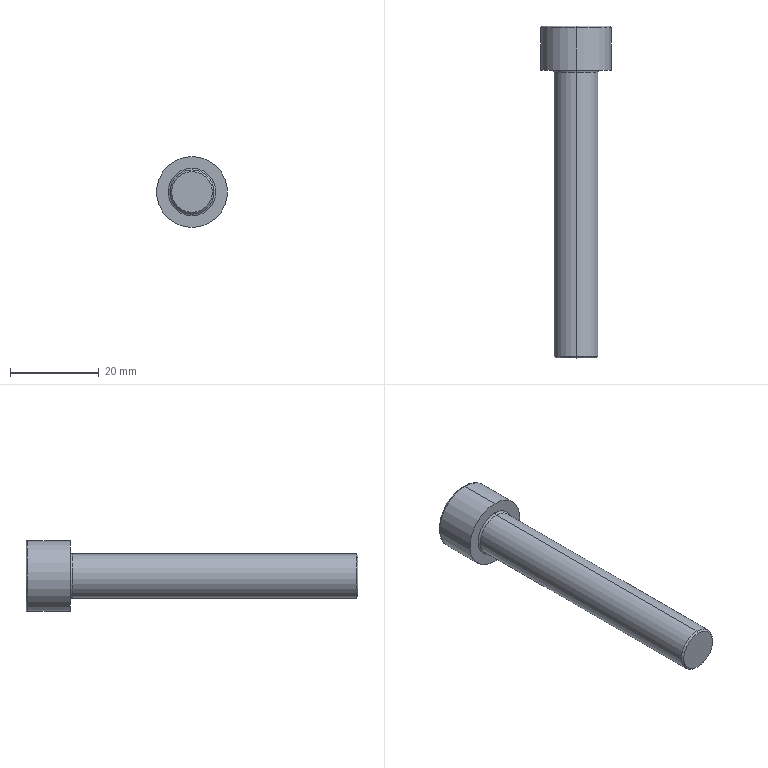Part | STEP file | 1 solid | 20 faces | box 16 x 75 x 16 mm | volume 6836 mm3 | plane 10 | torus 4 | cylinder 4 | cone 2 | commonest cylinder face diameters 10 x2 16 x2
STEP:
#1=CARTESIAN_POINT('',(0.,-65.,-4.6));
#2=VERTEX_POINT('',#1);
#3=CARTESIAN_POINT('',(0.,-65.,4.6));
#4=VERTEX_POINT('',#3);
#5=CARTESIAN_POINT('',(0.,-65.,0.));
#6=DIRECTION('',(0.,-1.,0.));
#7=DIRECTION('',(0.,0.,-1.));
#8=AXIS2_PLACEMENT_3D('',#5,#6,#7);
#9=CIRCLE('',#8,4.6);
#10=EDGE_CURVE('',#2,#4,#9,.T.);
#11=ORIENTED_EDGE('',*,*,#10,.F.);
#12=CARTESIAN_POINT('',(0.,-64.6,-5.));
#13=VERTEX_POINT('',#12);
#14=CARTESIAN_POINT('',(0.,-65.,-4.6));
#15=DIRECTION('',(0.,0.7071,-0.7071));
#16=VECTOR('',#15,1000.);
#17=LINE('',#14,#16);
#18=EDGE_CURVE('',#2,#13,#17,.T.);
#19=ORIENTED_EDGE('',*,*,#18,.T.);
#20=CARTESIAN_POINT('',(0.,-64.6,5.));
#21=VERTEX_POINT('',#20);
#22=CARTESIAN_POINT('',(0.,-64.6,0.));
#23=DIRECTION('',(0.,1.,0.));
#24=DIRECTION('',(0.,0.,-1.));
#25=AXIS2_PLACEMENT_3D('',#22,#23,#24);
#26=CIRCLE('',#25,5.);
#27=EDGE_CURVE('',#21,#13,#26,.T.);
#28=ORIENTED_EDGE('',*,*,#27,.F.);
#29=CARTESIAN_POINT('',(0.,-65.,4.6));
#30=DIRECTION('',(0.,0.7071,0.7071));
#31=VECTOR('',#30,1000.);
#32=LINE('',#29,#31);
#33=EDGE_CURVE('',#4,#21,#32,.T.);
#34=ORIENTED_EDGE('',*,*,#33,.F.);
#35=EDGE_LOOP('',(#11,#19,#28,#34));
#36=FACE_OUTER_BOUND('',#35,.T.);
#37=CARTESIAN_POINT('',(0.,-65.,0.));
#38=DIRECTION('',(0.,1.,0.));
#39=DIRECTION('',(0.,0.,1.));
#40=AXIS2_PLACEMENT_3D('',#37,#38,#39);
#41=CONICAL_SURFACE('',#40,4.6,0.7854);
#42=ADVANCED_FACE('',(#36),#41,.T.);
#43=CARTESIAN_POINT('',(0.,9.6,-8.));
#44=VERTEX_POINT('',#43);
#45=CARTESIAN_POINT('',(0.,9.6,8.));
#46=VERTEX_POINT('',#45);
#47=CARTESIAN_POINT('',(0.,9.6,0.));
#48=DIRECTION('',(0.,-1.,0.));
#49=DIRECTION('',(0.,0.,1.));
#50=AXIS2_PLACEMENT_3D('',#47,#48,#49);
#51=CIRCLE('',#50,8.);
#52=EDGE_CURVE('',#44,#46,#51,.T.);
#53=ORIENTED_EDGE('',*,*,#52,.F.);
#54=CARTESIAN_POINT('',(0.,10.,-7.6));
#55=VERTEX_POINT('',#54);
#56=CARTESIAN_POINT('',(0.,9.6,-7.6));
#57=DIRECTION('',(1.,0.,0.));
#58=DIRECTION('',(0.,0.,-1.));
#59=AXIS2_PLACEMENT_3D('',#56,#57,#58);
#60=CIRCLE('',#59,0.4);
#61=EDGE_CURVE('',#44,#55,#60,.T.);
#62=ORIENTED_EDGE('',*,*,#61,.T.);
#63=CARTESIAN_POINT('',(0.,10.,7.6));
#64=VERTEX_POINT('',#63);
#65=CARTESIAN_POINT('',(0.,10.,0.));
#66=DIRECTION('',(0.,1.,0.));
#67=DIRECTION('',(0.,0.,1.));
#68=AXIS2_PLACEMENT_3D('',#65,#66,#67);
#69=CIRCLE('',#68,7.6);
#70=EDGE_CURVE('',#64,#55,#69,.T.);
#71=ORIENTED_EDGE('',*,*,#70,.F.);
#72=CARTESIAN_POINT('',(0.,9.6,7.6));
#73=DIRECTION('',(-1.,0.,0.));
#74=DIRECTION('',(0.,0.,1.));
#75=AXIS2_PLACEMENT_3D('',#72,#73,#74);
#76=CIRCLE('',#75,0.4);
#77=EDGE_CURVE('',#46,#64,#76,.T.);
#78=ORIENTED_EDGE('',*,*,#77,.F.);
#79=EDGE_LOOP('',(#53,#62,#71,#78));
#80=FACE_OUTER_BOUND('',#79,.T.);
#81=CARTESIAN_POINT('',(0.,9.6,0.));
#82=DIRECTION('',(0.,1.,0.));
#83=DIRECTION('',(0.,0.,1.));
#84=AXIS2_PLACEMENT_3D('',#81,#82,#83);
#85=TOROIDAL_SURFACE('',#84,7.6,0.4);
#86=ADVANCED_FACE('',(#80),#85,.T.);
#87=CARTESIAN_POINT('',(0.,-0.4,5.));
#88=VERTEX_POINT('',#87);
#89=CARTESIAN_POINT('',(0.,-0.4,-5.));
#90=VERTEX_POINT('',#89);
#91=CARTESIAN_POINT('',(0.,-0.4,0.));
#92=DIRECTION('',(0.,-1.,0.));
#93=DIRECTION('',(0.,0.,-1.));
#94=AXIS2_PLACEMENT_3D('',#91,#92,#93);
#95=CIRCLE('',#94,5.);
#96=EDGE_CURVE('',#88,#90,#95,.T.);
#97=ORIENTED_EDGE('',*,*,#96,.F.);
#98=CARTESIAN_POINT('',(0.,0.,5.4));
#99=VERTEX_POINT('',#98);
#100=CARTESIAN_POINT('',(0.,-0.4,5.4));
#101=DIRECTION('',(1.,0.,0.));
#102=DIRECTION('',(0.,0.,-1.));
#103=AXIS2_PLACEMENT_3D('',#100,#101,#102);
#104=CIRCLE('',#103,0.4);
#105=EDGE_CURVE('',#88,#99,#104,.T.);
#106=ORIENTED_EDGE('',*,*,#105,.T.);
#107=CARTESIAN_POINT('',(0.,0.,-5.4));
#108=VERTEX_POINT('',#107);
#109=CARTESIAN_POINT('',(0.,0.,0.));
#110=DIRECTION('',(0.,1.,0.));
#111=DIRECTION('',(0.,0.,-1.));
#112=AXIS2_PLACEMENT_3D('',#109,#110,#111);
#113=CIRCLE('',#112,5.4);
#114=EDGE_CURVE('',#108,#99,#113,.T.);
#115=ORIENTED_EDGE('',*,*,#114,.F.);
#116=CARTESIAN_POINT('',(0.,-0.4,-5.4));
#117=DIRECTION('',(-1.,0.,0.));
#118=DIRECTION('',(0.,0.,1.));
#119=AXIS2_PLACEMENT_3D('',#116,#117,#118);
#120=CIRCLE('',#119,0.4);
#121=EDGE_CURVE('',#90,#108,#120,.T.);
#122=ORIENTED_EDGE('',*,*,#121,.F.);
#123=EDGE_LOOP('',(#97,#106,#115,#122));
#124=FACE_OUTER_BOUND('',#123,.T.);
#125=CARTESIAN_POINT('',(0.,-0.4,0.));
#126=DIRECTION('',(0.,-1.,0.));
#127=DIRECTION('',(0.,0.,-1.));
#128=AXIS2_PLACEMENT_3D('',#125,#126,#127);
#129=TOROIDAL_SURFACE('',#128,5.4,0.4);
#130=ADVANCED_FACE('',(#124),#129,.F.);
#131=CARTESIAN_POINT('',(0.,-0.4,0.));
#132=DIRECTION('',(0.,-1.,0.));
#133=DIRECTION('',(0.,0.,-1.));
#134=AXIS2_PLACEMENT_3D('',#131,#132,#133);
#135=CIRCLE('',#134,5.);
#136=EDGE_CURVE('',#90,#88,#135,.T.);
#137=ORIENTED_EDGE('',*,*,#136,.T.);
#138=CARTESIAN_POINT('',(0.,0.,5.));
#139=DIRECTION('',(0.,-1.,0.));
#140=VECTOR('',#139,1000.);
#141=LINE('',#138,#140);
#142=EDGE_CURVE('',#88,#21,#141,.T.);
#143=ORIENTED_EDGE('',*,*,#142,.T.);
#144=ORIENTED_EDGE('',*,*,#27,.T.);
#145=CARTESIAN_POINT('',(0.,0.,-5.));
#146=DIRECTION('',(0.,-1.,0.));
#147=VECTOR('',#146,1000.);
#148=LINE('',#145,#147);
#149=EDGE_CURVE('',#90,#13,#148,.T.);
#150=ORIENTED_EDGE('',*,*,#149,.F.);
#151=EDGE_LOOP('',(#137,#143,#144,#150));
#152=FACE_OUTER_BOUND('',#151,.T.);
#153=CARTESIAN_POINT('',(0.,0.,0.));
#154=DIRECTION('',(0.,-1.,0.));
#155=DIRECTION('',(0.,0.,-1.));
#156=AXIS2_PLACEMENT_3D('',#153,#154,#155);
#157=CYLINDRICAL_SURFACE('',#156,5.);
#158=ADVANCED_FACE('',(#152),#157,.T.);
#159=ORIENTED_EDGE('',*,*,#52,.T.);
#160=CARTESIAN_POINT('',(0.,0.,8.));
#161=VERTEX_POINT('',#160);
#162=CARTESIAN_POINT('',(0.,0.,8.));
#163=DIRECTION('',(0.,-1.,0.));
#164=VECTOR('',#163,1000.);
#165=LINE('',#162,#164);
#166=EDGE_CURVE('',#46,#161,#165,.T.);
#167=ORIENTED_EDGE('',*,*,#166,.T.);
#168=CARTESIAN_POINT('',(0.,0.,-8.));
#169=VERTEX_POINT('',#168);
#170=CARTESIAN_POINT('',(0.,0.,0.));
#171=DIRECTION('',(0.,-1.,0.));
#172=DIRECTION('',(0.,0.,-1.));
#173=AXIS2_PLACEMENT_3D('',#170,#171,#172);
#174=CIRCLE('',#173,8.);
#175=EDGE_CURVE('',#169,#161,#174,.T.);
#176=ORIENTED_EDGE('',*,*,#175,.F.);
#177=CARTESIAN_POINT('',(0.,0.,-8.));
#178=DIRECTION('',(0.,-1.,0.));
#179=VECTOR('',#178,1000.);
#180=LINE('',#177,#179);
#181=EDGE_CURVE('',#44,#169,#180,.T.);
#182=ORIENTED_EDGE('',*,*,#181,.F.);
#183=EDGE_LOOP('',(#159,#167,#176,#182));
#184=FACE_OUTER_BOUND('',#183,.T.);
#185=CARTESIAN_POINT('',(0.,0.,0.));
#186=DIRECTION('',(0.,-1.,0.));
#187=DIRECTION('',(0.,0.,-1.));
#188=AXIS2_PLACEMENT_3D('',#185,#186,#187);
#189=CYLINDRICAL_SURFACE('',#188,8.);
#190=ADVANCED_FACE('',(#184),#189,.T.);
#191=ORIENTED_EDGE('',*,*,#70,.T.);
#192=CARTESIAN_POINT('',(0.,10.,0.));
#193=DIRECTION('',(0.,1.,0.));
#194=DIRECTION('',(0.,0.,1.));
#195=AXIS2_PLACEMENT_3D('',#192,#193,#194);
#196=CIRCLE('',#195,7.6);
#197=EDGE_CURVE('',#55,#64,#196,.T.);
#198=ORIENTED_EDGE('',*,*,#197,.T.);
#199=EDGE_LOOP('',(#191,#198));
#200=FACE_OUTER_BOUND('',#199,.T.);
#201=CARTESIAN_POINT('',(0.,10.,-4.619));
#202=VERTEX_POINT('',#201);
#203=CARTESIAN_POINT('',(-4.,10.,-2.309));
#204=VERTEX_POINT('',#203);
#205=CARTESIAN_POINT('',(0.,10.,-4.619));
#206=DIRECTION('',(-0.866,0.,0.5));
#207=VECTOR('',#206,1000.);
#208=LINE('',#205,#207);
#209=EDGE_CURVE('',#202,#204,#208,.T.);
#210=ORIENTED_EDGE('',*,*,#209,.F.);
#211=CARTESIAN_POINT('',(4.,10.,-2.309));
#212=VERTEX_POINT('',#211);
#213=CARTESIAN_POINT('',(4.,10.,-2.309));
#214=DIRECTION('',(-0.866,0.,-0.5));
#215=VECTOR('',#214,1000.);
#216=LINE('',#213,#215);
#217=EDGE_CURVE('',#212,#202,#216,.T.);
#218=ORIENTED_EDGE('',*,*,#217,.F.);
#219=CARTESIAN_POINT('',(4.,10.,2.309));
#220=VERTEX_POINT('',#219);
#221=CARTESIAN_POINT('',(4.,10.,2.309));
#222=DIRECTION('',(0.,0.,-1.));
#223=VECTOR('',#222,1000.);
#224=LINE('',#221,#223);
#225=EDGE_CURVE('',#220,#212,#224,.T.);
#226=ORIENTED_EDGE('',*,*,#225,.F.);
#227=CARTESIAN_POINT('',(0.,10.,4.619));
#228=VERTEX_POINT('',#227);
#229=CARTESIAN_POINT('',(0.,10.,4.619));
#230=DIRECTION('',(0.866,0.,-0.5));
#231=VECTOR('',#230,1000.);
#232=LINE('',#229,#231);
#233=EDGE_CURVE('',#228,#220,#232,.T.);
#234=ORIENTED_EDGE('',*,*,#233,.F.);
#235=CARTESIAN_POINT('',(-4.,10.,2.309));
#236=VERTEX_POINT('',#235);
#237=CARTESIAN_POINT('',(-4.,10.,2.309));
#238=DIRECTION('',(0.866,0.,0.5));
#239=VECTOR('',#238,1000.);
#240=LINE('',#237,#239);
#241=EDGE_CURVE('',#236,#228,#240,.T.);
#242=ORIENTED_EDGE('',*,*,#241,.F.);
#243=CARTESIAN_POINT('',(-4.,10.,-2.309));
#244=DIRECTION('',(0.,0.,1.));
#245=VECTOR('',#244,1000.);
#246=LINE('',#243,#245);
#247=EDGE_CURVE('',#204,#236,#246,.T.);
#248=ORIENTED_EDGE('',*,*,#247,.F.);
#249=EDGE_LOOP('',(#210,#218,#226,#234,#242,#248));
#250=FACE_BOUND('',#249,.T.);
#251=CARTESIAN_POINT('',(0.,10.,0.));
#252=DIRECTION('',(0.,1.,0.));
#253=DIRECTION('',(0.,0.,1.));
#254=AXIS2_PLACEMENT_3D('',#251,#252,#253);
#255=PLANE('',#254);
#256=ADVANCED_FACE('',(#200,#250),#255,.T.);
#257=ORIENTED_EDGE('',*,*,#166,.F.);
#258=CARTESIAN_POINT('',(0.,9.6,0.));
#259=DIRECTION('',(0.,-1.,0.));
#260=DIRECTION('',(0.,0.,1.));
#261=AXIS2_PLACEMENT_3D('',#258,#259,#260);
#262=CIRCLE('',#261,8.);
#263=EDGE_CURVE('',#46,#44,#262,.T.);
#264=ORIENTED_EDGE('',*,*,#263,.T.);
#265=ORIENTED_EDGE('',*,*,#181,.T.);
#266=CARTESIAN_POINT('',(0.,0.,0.));
#267=DIRECTION('',(0.,-1.,0.));
#268=DIRECTION('',(0.,0.,-1.));
#269=AXIS2_PLACEMENT_3D('',#266,#267,#268);
#270=CIRCLE('',#269,8.);
#271=EDGE_CURVE('',#161,#169,#270,.T.);
#272=ORIENTED_EDGE('',*,*,#271,.F.);
#273=EDGE_LOOP('',(#257,#264,#265,#272));
#274=FACE_OUTER_BOUND('',#273,.T.);
#275=CARTESIAN_POINT('',(0.,0.,0.));
#276=DIRECTION('',(0.,-1.,0.));
#277=DIRECTION('',(0.,0.,-1.));
#278=AXIS2_PLACEMENT_3D('',#275,#276,#277);
#279=CYLINDRICAL_SURFACE('',#278,8.);
#280=ADVANCED_FACE('',(#274),#279,.T.);
#281=ORIENTED_EDGE('',*,*,#114,.T.);
#282=CARTESIAN_POINT('',(0.,0.,0.));
#283=DIRECTION('',(0.,1.,0.));
#284=DIRECTION('',(0.,0.,-1.));
#285=AXIS2_PLACEMENT_3D('',#282,#283,#284);
#286=CIRCLE('',#285,5.4);
#287=EDGE_CURVE('',#99,#108,#286,.T.);
#288=ORIENTED_EDGE('',*,*,#287,.T.);
#289=EDGE_LOOP('',(#281,#288));
#290=FACE_BOUND('',#289,.T.);
#291=ORIENTED_EDGE('',*,*,#175,.T.);
#292=ORIENTED_EDGE('',*,*,#271,.T.);
#293=EDGE_LOOP('',(#291,#292));
#294=FACE_OUTER_BOUND('',#293,.T.);
#295=CARTESIAN_POINT('',(8.,0.,0.));
#296=DIRECTION('',(0.,-1.,0.));
#297=DIRECTION('',(0.,0.,-1.));
#298=AXIS2_PLACEMENT_3D('',#295,#296,#297);
#299=PLANE('',#298);
#300=ADVANCED_FACE('',(#290,#294),#299,.T.);
#301=ORIENTED_EDGE('',*,*,#142,.F.);
#302=ORIENTED_EDGE('',*,*,#96,.T.);
#303=ORIENTED_EDGE('',*,*,#149,.T.);
#304=CARTESIAN_POINT('',(0.,-64.6,0.));
#305=DIRECTION('',(0.,1.,0.));
#306=DIRECTION('',(0.,0.,-1.));
#307=AXIS2_PLACEMENT_3D('',#304,#305,#306);
#308=CIRCLE('',#307,5.);
#309=EDGE_CURVE('',#13,#21,#308,.T.);
#310=ORIENTED_EDGE('',*,*,#309,.T.);
#311=EDGE_LOOP('',(#301,#302,#303,#310));
#312=FACE_OUTER_BOUND('',#311,.T.);
#313=CARTESIAN_POINT('',(0.,0.,0.));
#314=DIRECTION('',(0.,-1.,0.));
#315=DIRECTION('',(0.,0.,-1.));
#316=AXIS2_PLACEMENT_3D('',#313,#314,#315);
#317=CYLINDRICAL_SURFACE('',#316,5.);
#318=ADVANCED_FACE('',(#312),#317,.T.);
#319=CARTESIAN_POINT('',(0.,-65.,0.));
#320=DIRECTION('',(0.,-1.,0.));
#321=DIRECTION('',(0.,0.,-1.));
#322=AXIS2_PLACEMENT_3D('',#319,#320,#321);
#323=CIRCLE('',#322,4.6);
#324=EDGE_CURVE('',#4,#2,#323,.T.);
#325=ORIENTED_EDGE('',*,*,#324,.T.);
#326=ORIENTED_EDGE('',*,*,#10,.T.);
#327=EDGE_LOOP('',(#325,#326));
#328=FACE_OUTER_BOUND('',#327,.T.);
#329=CARTESIAN_POINT('',(5.,-65.,0.));
#330=DIRECTION('',(0.,-1.,0.));
#331=DIRECTION('',(0.,0.,-1.));
#332=AXIS2_PLACEMENT_3D('',#329,#330,#331);
#333=PLANE('',#332);
#334=ADVANCED_FACE('',(#328),#333,.T.);
#335=ORIENTED_EDGE('',*,*,#209,.T.);
#336=CARTESIAN_POINT('',(-4.,5.,-2.309));
#337=VERTEX_POINT('',#336);
#338=CARTESIAN_POINT('',(-4.,5.,-2.309));
#339=DIRECTION('',(0.,1.,0.));
#340=VECTOR('',#339,1000.);
#341=LINE('',#338,#340);
#342=EDGE_CURVE('',#337,#204,#341,.T.);
#343=ORIENTED_EDGE('',*,*,#342,.F.);
#344=CARTESIAN_POINT('',(0.,5.,-4.619));
#345=VERTEX_POINT('',#344);
#346=CARTESIAN_POINT('',(0.,5.,-4.619));
#347=DIRECTION('',(-0.866,0.,0.5));
#348=VECTOR('',#347,1000.);
#349=LINE('',#346,#348);
#350=EDGE_CURVE('',#345,#337,#349,.T.);
#351=ORIENTED_EDGE('',*,*,#350,.F.);
#352=CARTESIAN_POINT('',(0.,5.,-4.619));
#353=DIRECTION('',(0.,1.,0.));
#354=VECTOR('',#353,1000.);
#355=LINE('',#352,#354);
#356=EDGE_CURVE('',#345,#202,#355,.T.);
#357=ORIENTED_EDGE('',*,*,#356,.T.);
#358=EDGE_LOOP('',(#335,#343,#351,#357));
#359=FACE_OUTER_BOUND('',#358,.T.);
#360=CARTESIAN_POINT('',(0.,5.,-4.619));
#361=DIRECTION('',(-0.5,0.,-0.866));
#362=DIRECTION('',(-0.866,0.,0.5));
#363=AXIS2_PLACEMENT_3D('',#360,#361,#362);
#364=PLANE('',#363);
#365=ADVANCED_FACE('',(#359),#364,.F.);
#366=ORIENTED_EDGE('',*,*,#217,.T.);
#367=ORIENTED_EDGE('',*,*,#356,.F.);
#368=CARTESIAN_POINT('',(4.,5.,-2.309));
#369=VERTEX_POINT('',#368);
#370=CARTESIAN_POINT('',(4.,5.,-2.309));
#371=DIRECTION('',(-0.866,0.,-0.5));
#372=VECTOR('',#371,1000.);
#373=LINE('',#370,#372);
#374=EDGE_CURVE('',#369,#345,#373,.T.);
#375=ORIENTED_EDGE('',*,*,#374,.F.);
#376=CARTESIAN_POINT('',(4.,5.,-2.309));
#377=DIRECTION('',(0.,1.,0.));
#378=VECTOR('',#377,1000.);
#379=LINE('',#376,#378);
#380=EDGE_CURVE('',#369,#212,#379,.T.);
#381=ORIENTED_EDGE('',*,*,#380,.T.);
#382=EDGE_LOOP('',(#366,#367,#375,#381));
#383=FACE_OUTER_BOUND('',#382,.T.);
#384=CARTESIAN_POINT('',(4.,5.,-2.309));
#385=DIRECTION('',(0.5,0.,-0.866));
#386=DIRECTION('',(-0.866,0.,-0.5));
#387=AXIS2_PLACEMENT_3D('',#384,#385,#386);
#388=PLANE('',#387);
#389=ADVANCED_FACE('',(#383),#388,.F.);
#390=ORIENTED_EDGE('',*,*,#225,.T.);
#391=ORIENTED_EDGE('',*,*,#380,.F.);
#392=CARTESIAN_POINT('',(4.,5.,2.309));
#393=VERTEX_POINT('',#392);
#394=CARTESIAN_POINT('',(4.,5.,2.309));
#395=DIRECTION('',(0.,0.,-1.));
#396=VECTOR('',#395,1000.);
#397=LINE('',#394,#396);
#398=EDGE_CURVE('',#393,#369,#397,.T.);
#399=ORIENTED_EDGE('',*,*,#398,.F.);
#400=CARTESIAN_POINT('',(4.,5.,2.309));
#401=DIRECTION('',(0.,1.,0.));
#402=VECTOR('',#401,1000.);
#403=LINE('',#400,#402);
#404=EDGE_CURVE('',#393,#220,#403,.T.);
#405=ORIENTED_EDGE('',*,*,#404,.T.);
#406=EDGE_LOOP('',(#390,#391,#399,#405));
#407=FACE_OUTER_BOUND('',#406,.T.);
#408=CARTESIAN_POINT('',(4.,5.,2.309));
#409=DIRECTION('',(1.,0.,0.));
#410=DIRECTION('',(0.,0.,-1.));
#411=AXIS2_PLACEMENT_3D('',#408,#409,#410);
#412=PLANE('',#411);
#413=ADVANCED_FACE('',(#407),#412,.F.);
#414=ORIENTED_EDGE('',*,*,#233,.T.);
#415=ORIENTED_EDGE('',*,*,#404,.F.);
#416=CARTESIAN_POINT('',(0.,5.,4.619));
#417=VERTEX_POINT('',#416);
#418=CARTESIAN_POINT('',(0.,5.,4.619));
#419=DIRECTION('',(0.866,0.,-0.5));
#420=VECTOR('',#419,1000.);
#421=LINE('',#418,#420);
#422=EDGE_CURVE('',#417,#393,#421,.T.);
#423=ORIENTED_EDGE('',*,*,#422,.F.);
#424=CARTESIAN_POINT('',(0.,5.,4.619));
#425=DIRECTION('',(0.,1.,0.));
#426=VECTOR('',#425,1000.);
#427=LINE('',#424,#426);
#428=EDGE_CURVE('',#417,#228,#427,.T.);
#429=ORIENTED_EDGE('',*,*,#428,.T.);
#430=EDGE_LOOP('',(#414,#415,#423,#429));
#431=FACE_OUTER_BOUND('',#430,.T.);
#432=CARTESIAN_POINT('',(0.,5.,4.619));
#433=DIRECTION('',(0.5,0.,0.866));
#434=DIRECTION('',(0.866,0.,-0.5));
#435=AXIS2_PLACEMENT_3D('',#432,#433,#434);
#436=PLANE('',#435);
#437=ADVANCED_FACE('',(#431),#436,.F.);
#438=ORIENTED_EDGE('',*,*,#241,.T.);
#439=ORIENTED_EDGE('',*,*,#428,.F.);
#440=CARTESIAN_POINT('',(-4.,5.,2.309));
#441=VERTEX_POINT('',#440);
#442=CARTESIAN_POINT('',(-4.,5.,2.309));
#443=DIRECTION('',(0.866,0.,0.5));
#444=VECTOR('',#443,1000.);
#445=LINE('',#442,#444);
#446=EDGE_CURVE('',#441,#417,#445,.T.);
#447=ORIENTED_EDGE('',*,*,#446,.F.);
#448=CARTESIAN_POINT('',(-4.,5.,2.309));
#449=DIRECTION('',(0.,1.,0.));
#450=VECTOR('',#449,1000.);
#451=LINE('',#448,#450);
#452=EDGE_CURVE('',#441,#236,#451,.T.);
#453=ORIENTED_EDGE('',*,*,#452,.T.);
#454=EDGE_LOOP('',(#438,#439,#447,#453));
#455=FACE_OUTER_BOUND('',#454,.T.);
#456=CARTESIAN_POINT('',(-4.,5.,2.309));
#457=DIRECTION('',(-0.5,0.,0.866));
#458=DIRECTION('',(0.866,0.,0.5));
#459=AXIS2_PLACEMENT_3D('',#456,#457,#458);
#460=PLANE('',#459);
#461=ADVANCED_FACE('',(#455),#460,.F.);
#462=ORIENTED_EDGE('',*,*,#247,.T.);
#463=ORIENTED_EDGE('',*,*,#452,.F.);
#464=CARTESIAN_POINT('',(-4.,5.,-2.309));
#465=DIRECTION('',(0.,0.,1.));
#466=VECTOR('',#465,1000.);
#467=LINE('',#464,#466);
#468=EDGE_CURVE('',#337,#441,#467,.T.);
#469=ORIENTED_EDGE('',*,*,#468,.F.);
#470=ORIENTED_EDGE('',*,*,#342,.T.);
#471=EDGE_LOOP('',(#462,#463,#469,#470));
#472=FACE_OUTER_BOUND('',#471,.T.);
#473=CARTESIAN_POINT('',(-4.,5.,-2.309));
#474=DIRECTION('',(-1.,0.,0.));
#475=DIRECTION('',(0.,0.,1.));
#476=AXIS2_PLACEMENT_3D('',#473,#474,#475);
#477=PLANE('',#476);
#478=ADVANCED_FACE('',(#472),#477,.F.);
#479=ORIENTED_EDGE('',*,*,#350,.T.);
#480=ORIENTED_EDGE('',*,*,#468,.T.);
#481=ORIENTED_EDGE('',*,*,#446,.T.);
#482=ORIENTED_EDGE('',*,*,#422,.T.);
#483=ORIENTED_EDGE('',*,*,#398,.T.);
#484=ORIENTED_EDGE('',*,*,#374,.T.);
#485=EDGE_LOOP('',(#479,#480,#481,#482,#483,#484));
#486=FACE_OUTER_BOUND('',#485,.T.);
#487=CARTESIAN_POINT('',(0.,5.,0.));
#488=DIRECTION('',(0.,1.,0.));
#489=DIRECTION('',(0.,0.,1.));
#490=AXIS2_PLACEMENT_3D('',#487,#488,#489);
#491=PLANE('',#490);
#492=ADVANCED_FACE('',(#486),#491,.T.);
#493=ORIENTED_EDGE('',*,*,#105,.F.);
#494=ORIENTED_EDGE('',*,*,#136,.F.);
#495=ORIENTED_EDGE('',*,*,#121,.T.);
#496=ORIENTED_EDGE('',*,*,#287,.F.);
#497=EDGE_LOOP('',(#493,#494,#495,#496));
#498=FACE_OUTER_BOUND('',#497,.T.);
#499=CARTESIAN_POINT('',(0.,-0.4,0.));
#500=DIRECTION('',(0.,-1.,0.));
#501=DIRECTION('',(0.,0.,-1.));
#502=AXIS2_PLACEMENT_3D('',#499,#500,#501);
#503=TOROIDAL_SURFACE('',#502,5.4,0.4);
#504=ADVANCED_FACE('',(#498),#503,.F.);
#505=ORIENTED_EDGE('',*,*,#61,.F.);
#506=ORIENTED_EDGE('',*,*,#263,.F.);
#507=ORIENTED_EDGE('',*,*,#77,.T.);
#508=ORIENTED_EDGE('',*,*,#197,.F.);
#509=EDGE_LOOP('',(#505,#506,#507,#508));
#510=FACE_OUTER_BOUND('',#509,.T.);
#511=CARTESIAN_POINT('',(0.,9.6,0.));
#512=DIRECTION('',(0.,1.,0.));
#513=DIRECTION('',(0.,0.,1.));
#514=AXIS2_PLACEMENT_3D('',#511,#512,#513);
#515=TOROIDAL_SURFACE('',#514,7.6,0.4);
#516=ADVANCED_FACE('',(#510),#515,.T.);
#517=ORIENTED_EDGE('',*,*,#18,.F.);
#518=ORIENTED_EDGE('',*,*,#324,.F.);
#519=ORIENTED_EDGE('',*,*,#33,.T.);
#520=ORIENTED_EDGE('',*,*,#309,.F.);
#521=EDGE_LOOP('',(#517,#518,#519,#520));
#522=FACE_OUTER_BOUND('',#521,.T.);
#523=CARTESIAN_POINT('',(0.,-65.,0.));
#524=DIRECTION('',(0.,1.,0.));
#525=DIRECTION('',(0.,0.,1.));
#526=AXIS2_PLACEMENT_3D('',#523,#524,#525);
#527=CONICAL_SURFACE('',#526,4.6,0.7854);
#528=ADVANCED_FACE('',(#522),#527,.T.);
#529=CLOSED_SHELL('',(#42,#86,#130,#158,#190,#256,#280,#300,#318,#334,#365,#389,#413,#437,#461,#478,#492,#504,#516,#528));
#530=MANIFOLD_SOLID_BREP('',#529);
#531=CARTESIAN_POINT('',(0.,0.,0.));
#532=DIRECTION('',(0.,0.,1.));
#533=DIRECTION('',(1.,0.,0.));
#534=AXIS2_PLACEMENT_3D('',#531,#532,#533);
#535=(LENGTH_UNIT()NAMED_UNIT(*)SI_UNIT(.MILLI.,.METRE.));
#536=UNCERTAINTY_MEASURE_WITH_UNIT(LENGTH_MEASURE(0.00001),#535,'','');
#537=(NAMED_UNIT(*)PLANE_ANGLE_UNIT()SI_UNIT($,.RADIAN.));
#538=(NAMED_UNIT(*)SI_UNIT($,.STERADIAN.)SOLID_ANGLE_UNIT());
#539=(GEOMETRIC_REPRESENTATION_CONTEXT(3)GLOBAL_UNCERTAINTY_ASSIGNED_CONTEXT((#536))GLOBAL_UNIT_ASSIGNED_CONTEXT((#535,#537,#538))REPRESENTATION_CONTEXT('',''));
#540=ADVANCED_BREP_SHAPE_REPRESENTATION('',(#530,#534),#539);